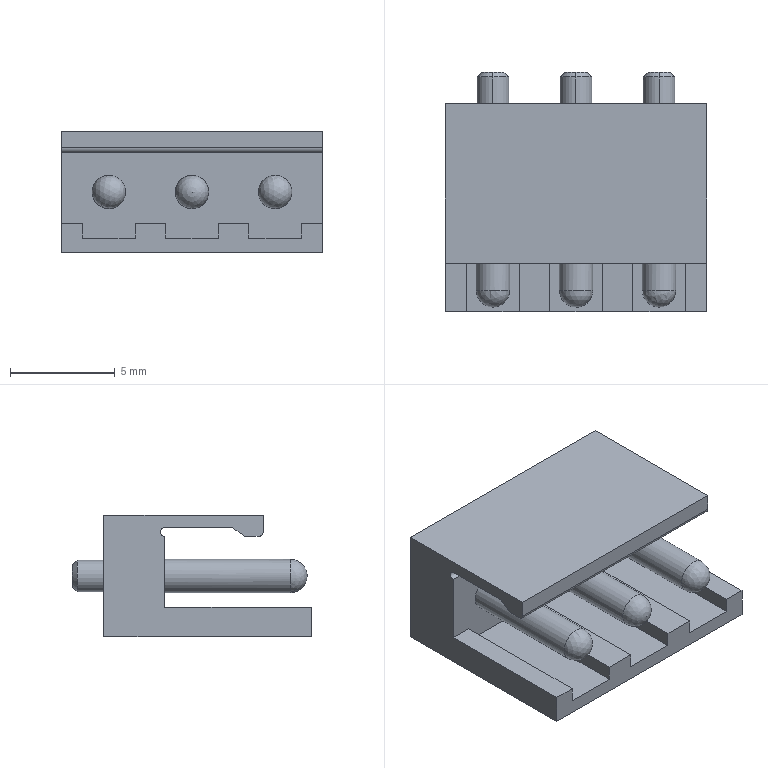Part | STEP file | JL27-03ZJB | 1 solid | 47 faces | box 12.48 x 11.4 x 5.8 mm | volume 382.21 mm3 | plane 27 | cylinder 11 | cone 6 | sphere 3 | commonest cylinder face diameters 1.5 x6 1.59 x3 0.4 x2